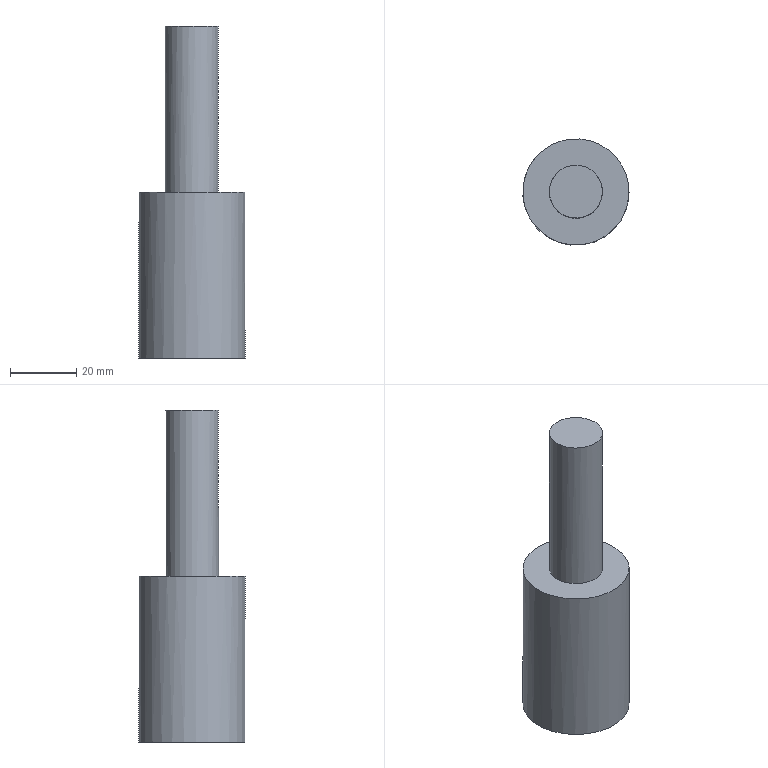Part | NX | features solid 2 | 1 solid | 7 faces | box 32 x 32 x 100 mm | volume 46984 mm3 | cylinder 3 | plane 3 | spline 1 | commonest cylinder face diameters 12 x1 16 x1 32 x1
STEP:
#1=CARTESIAN_POINT('',(678.834,-88.038,-30.));
#2=VERTEX_POINT('',#1);
#3=CARTESIAN_POINT('',(674.936,-93.067,-30.));
#4=CARTESIAN_POINT('',(680.633,-86.642,-30.));
#5=CARTESIAN_POINT('',(682.136,-75.462,-30.));
#6=CARTESIAN_POINT('',(673.917,-64.675,-30.));
#7=CARTESIAN_POINT('',(660.467,-62.856,-30.));
#8=CARTESIAN_POINT('',(649.671,-71.089,-30.));
#9=CARTESIAN_POINT('',(647.859,-84.528,-30.));
#10=CARTESIAN_POINT('',(654.704,-93.503,-30.));
#11=CARTESIAN_POINT('',(662.804,-96.267,-30.));
#12=CARTESIAN_POINT('',(669.194,-95.871,-30.));
#13=CARTESIAN_POINT('',(674.936,-93.067,-30.));
#14=CARTESIAN_POINT('',(680.633,-86.642,-30.));
#15=CARTESIAN_POINT('',(682.136,-75.462,-30.));
#16=B_SPLINE_CURVE_WITH_KNOTS('',3,(#3,#4,#5,#6,#7,#8,#9,#10,#11,#12,#13,#14,#15),.UNSPECIFIED.,.T.,.F.,(1,1,1,1,1,1,1,1,1,1,1,1,1,1,1,1,1),(-0.01876,-0.0125,-0.006252,0.,0.0125,0.02501,0.03751,0.05002,0.06252,0.07503,0.08128,0.08753,0.09378,0.1,0.1125,0.125,0.1375),.UNSPECIFIED.);
#17=EDGE_CURVE('',#2,#2,#16,.T.);
#18=ORIENTED_EDGE('',*,*,#17,.T.);
#19=EDGE_LOOP('',(#18));
#20=FACE_BOUND('',#19,.T.);
#21=CARTESIAN_POINT('',(657.,-80.,-30.));
#22=VERTEX_POINT('',#21);
#23=CARTESIAN_POINT('',(658.736,-86.276,-30.));
#24=CARTESIAN_POINT('',(656.133,-79.998,-30.));
#25=CARTESIAN_POINT('',(658.734,-73.73,-30.));
#26=CARTESIAN_POINT('',(664.994,-71.136,-30.));
#27=CARTESIAN_POINT('',(671.266,-73.727,-30.));
#28=CARTESIAN_POINT('',(673.865,-79.999,-30.));
#29=CARTESIAN_POINT('',(671.275,-86.261,-30.));
#30=CARTESIAN_POINT('',(665.01,-88.866,-30.));
#31=CARTESIAN_POINT('',(658.736,-86.276,-30.));
#32=CARTESIAN_POINT('',(656.133,-79.998,-30.));
#33=CARTESIAN_POINT('',(658.734,-73.73,-30.));
#34=B_SPLINE_CURVE_WITH_KNOTS('',3,(#23,#24,#25,#26,#27,#28,#29,#30,#31,#32,#33),.UNSPECIFIED.,.T.,.F.,(1,1,1,1,1,1,1,1,1,1,1,1,1,1,1),(-0.01876,-0.0125,-0.006252,0.,0.006252,0.0125,0.01876,0.02501,0.03126,0.03751,0.04377,0.05002,0.05627,0.06252,0.06877),.UNSPECIFIED.);
#35=EDGE_CURVE('',#22,#22,#34,.T.);
#36=ORIENTED_EDGE('',*,*,#35,.T.);
#37=EDGE_LOOP('',(#36));
#38=FACE_BOUND('',#37,.T.);
#39=CARTESIAN_POINT('',(648.808,-96.192,-30.));
#40=CARTESIAN_POINT('',(648.808,-85.397,-30.));
#41=CARTESIAN_POINT('',(648.808,-74.603,-30.));
#42=CARTESIAN_POINT('',(648.808,-63.808,-30.));
#43=CARTESIAN_POINT('',(659.603,-96.192,-30.));
#44=CARTESIAN_POINT('',(659.603,-85.397,-30.));
#45=CARTESIAN_POINT('',(659.603,-74.603,-30.));
#46=CARTESIAN_POINT('',(659.603,-63.808,-30.));
#47=CARTESIAN_POINT('',(670.397,-96.192,-30.));
#48=CARTESIAN_POINT('',(670.397,-85.397,-30.));
#49=CARTESIAN_POINT('',(670.397,-74.603,-30.));
#50=CARTESIAN_POINT('',(670.397,-63.808,-30.));
#51=CARTESIAN_POINT('',(681.192,-96.192,-30.));
#52=CARTESIAN_POINT('',(681.192,-85.397,-30.));
#53=CARTESIAN_POINT('',(681.192,-74.603,-30.));
#54=CARTESIAN_POINT('',(681.192,-63.808,-30.));
#55=B_SPLINE_SURFACE_WITH_KNOTS('',3,3,((#39,#40,#41,#42),(#43,#44,#45,#46),(#47,#48,#49,#50),(#51,#52,#53,#54)),.UNSPECIFIED.,.F.,.F.,.F.,(4,4),(4,4),(0.,1.),(0.,1.),.UNSPECIFIED.);
#56=ADVANCED_FACE('',(#20,#38),#55,.T.);
#57=CARTESIAN_POINT('',(681.,-80.,-80.));
#58=VERTEX_POINT('',#57);
#59=CARTESIAN_POINT('',(665.,-80.,-80.));
#60=DIRECTION('',(0.,0.,1.));
#61=DIRECTION('',(1.,0.,0.));
#62=AXIS2_PLACEMENT_3D('',#59,#60,#61);
#63=CIRCLE('',#62,16.);
#64=EDGE_CURVE('',#58,#58,#63,.T.);
#65=ORIENTED_EDGE('',*,*,#64,.T.);
#66=EDGE_LOOP('',(#65));
#67=FACE_BOUND('',#66,.T.);
#68=ORIENTED_EDGE('',*,*,#17,.F.);
#69=EDGE_LOOP('',(#68));
#70=FACE_BOUND('',#69,.T.);
#71=CARTESIAN_POINT('',(665.,-80.,-2.));
#72=DIRECTION('',(0.,0.,-1.));
#73=DIRECTION('',(-1.,0.,0.));
#74=AXIS2_PLACEMENT_3D('',#71,#72,#73);
#75=CYLINDRICAL_SURFACE('',#74,16.);
#76=ADVANCED_FACE('',(#67,#70),#75,.T.);
#77=ORIENTED_EDGE('',*,*,#64,.F.);
#78=EDGE_LOOP('',(#77));
#79=FACE_BOUND('',#78,.T.);
#80=CARTESIAN_POINT('',(671.,-80.,-80.));
#81=VERTEX_POINT('',#80);
#82=CARTESIAN_POINT('',(665.,-80.,-80.));
#83=DIRECTION('',(0.,0.,1.));
#84=DIRECTION('',(1.,0.,0.));
#85=AXIS2_PLACEMENT_3D('',#82,#83,#84);
#86=CIRCLE('',#85,6.);
#87=EDGE_CURVE('',#81,#81,#86,.T.);
#88=ORIENTED_EDGE('',*,*,#87,.T.);
#89=EDGE_LOOP('',(#88));
#90=FACE_BOUND('',#89,.T.);
#91=CARTESIAN_POINT('',(665.,-80.,-80.));
#92=DIRECTION('',(0.,0.,1.));
#93=DIRECTION('',(1.,0.,0.));
#94=AXIS2_PLACEMENT_3D('',#91,#92,#93);
#95=PLANE('',#94);
#96=ADVANCED_FACE('',(#79,#90),#95,.F.);
#97=CARTESIAN_POINT('',(671.,-80.,-51.));
#98=VERTEX_POINT('',#97);
#99=CARTESIAN_POINT('',(665.,-80.,-51.));
#100=DIRECTION('',(0.,0.,1.));
#101=DIRECTION('',(1.,0.,0.));
#102=AXIS2_PLACEMENT_3D('',#99,#100,#101);
#103=CIRCLE('',#102,6.);
#104=EDGE_CURVE('',#98,#98,#103,.T.);
#105=ORIENTED_EDGE('',*,*,#104,.F.);
#106=EDGE_LOOP('',(#105));
#107=FACE_BOUND('',#106,.T.);
#108=CARTESIAN_POINT('',(665.,-80.,-51.));
#109=DIRECTION('',(0.,0.,1.));
#110=DIRECTION('',(-1.,0.,0.));
#111=AXIS2_PLACEMENT_3D('',#108,#109,#110);
#112=PLANE('',#111);
#113=ADVANCED_FACE('',(#107),#112,.F.);
#114=ORIENTED_EDGE('',*,*,#87,.F.);
#115=EDGE_LOOP('',(#114));
#116=FACE_BOUND('',#115,.T.);
#117=ORIENTED_EDGE('',*,*,#104,.T.);
#118=EDGE_LOOP('',(#117));
#119=FACE_BOUND('',#118,.T.);
#120=CARTESIAN_POINT('',(665.,-80.,-81.));
#121=DIRECTION('',(0.,0.,-1.));
#122=DIRECTION('',(1.,0.,0.));
#123=AXIS2_PLACEMENT_3D('',#120,#121,#122);
#124=CYLINDRICAL_SURFACE('',#123,6.);
#125=ADVANCED_FACE('',(#116,#119),#124,.F.);
#126=CARTESIAN_POINT('',(673.,-80.,20.));
#127=VERTEX_POINT('',#126);
#128=CARTESIAN_POINT('',(665.,-80.,20.));
#129=DIRECTION('',(0.,0.,1.));
#130=DIRECTION('',(1.,0.,0.));
#131=AXIS2_PLACEMENT_3D('',#128,#129,#130);
#132=CIRCLE('',#131,8.);
#133=EDGE_CURVE('',#127,#127,#132,.T.);
#134=ORIENTED_EDGE('',*,*,#133,.T.);
#135=EDGE_LOOP('',(#134));
#136=FACE_BOUND('',#135,.T.);
#137=CARTESIAN_POINT('',(665.,-80.,20.));
#138=DIRECTION('',(0.,0.,1.));
#139=DIRECTION('',(1.,0.,0.));
#140=AXIS2_PLACEMENT_3D('',#137,#138,#139);
#141=PLANE('',#140);
#142=ADVANCED_FACE('',(#136),#141,.T.);
#143=ORIENTED_EDGE('',*,*,#35,.F.);
#144=EDGE_LOOP('',(#143));
#145=FACE_BOUND('',#144,.T.);
#146=ORIENTED_EDGE('',*,*,#133,.F.);
#147=EDGE_LOOP('',(#146));
#148=FACE_BOUND('',#147,.T.);
#149=CARTESIAN_POINT('',(665.,-80.,-2.));
#150=DIRECTION('',(0.,0.,-1.));
#151=DIRECTION('',(-1.,0.,0.));
#152=AXIS2_PLACEMENT_3D('',#149,#150,#151);
#153=CYLINDRICAL_SURFACE('',#152,8.);
#154=ADVANCED_FACE('',(#145,#148),#153,.T.);
#155=CLOSED_SHELL('',(#56,#76,#96,#113,#125,#142,#154));
#156=MANIFOLD_SOLID_BREP('',#155);
#157=(LENGTH_UNIT()NAMED_UNIT(*)SI_UNIT(.MILLI.,.METRE.));
#158=UNCERTAINTY_MEASURE_WITH_UNIT(LENGTH_MEASURE(0.0508),#157,'','');
#159=(NAMED_UNIT(*)PLANE_ANGLE_UNIT()SI_UNIT($,.RADIAN.));
#160=(NAMED_UNIT(*)SI_UNIT($,.STERADIAN.)SOLID_ANGLE_UNIT());
#161=(GEOMETRIC_REPRESENTATION_CONTEXT(3)GLOBAL_UNCERTAINTY_ASSIGNED_CONTEXT((#158))GLOBAL_UNIT_ASSIGNED_CONTEXT((#157,#159,#160))REPRESENTATION_CONTEXT('',''));
#162=ADVANCED_BREP_SHAPE_REPRESENTATION('',(#156),#161);